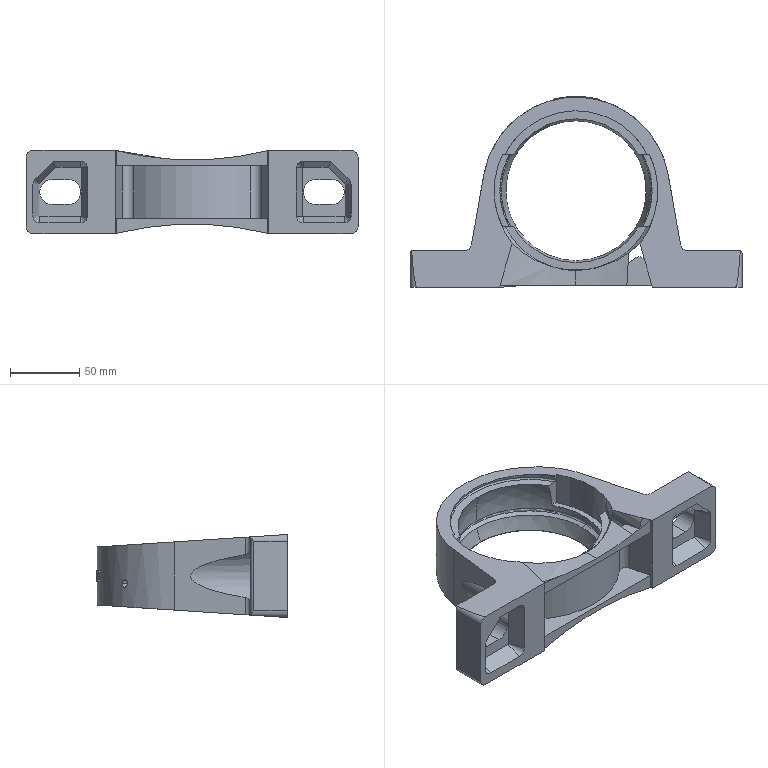Part | SolidWorks | features BaseBody 1 | 1 solid | 235 faces | box 240 x 138 x 60 mm | volume 436928 mm3 | plane 106 | cylinder 91 | cone 22 | torus 10 | sphere 6 | commonest cylinder face diameters 0.242 x14 0.416 x14 0.769 x13 0.236 x10 10 x10 115.323 x6